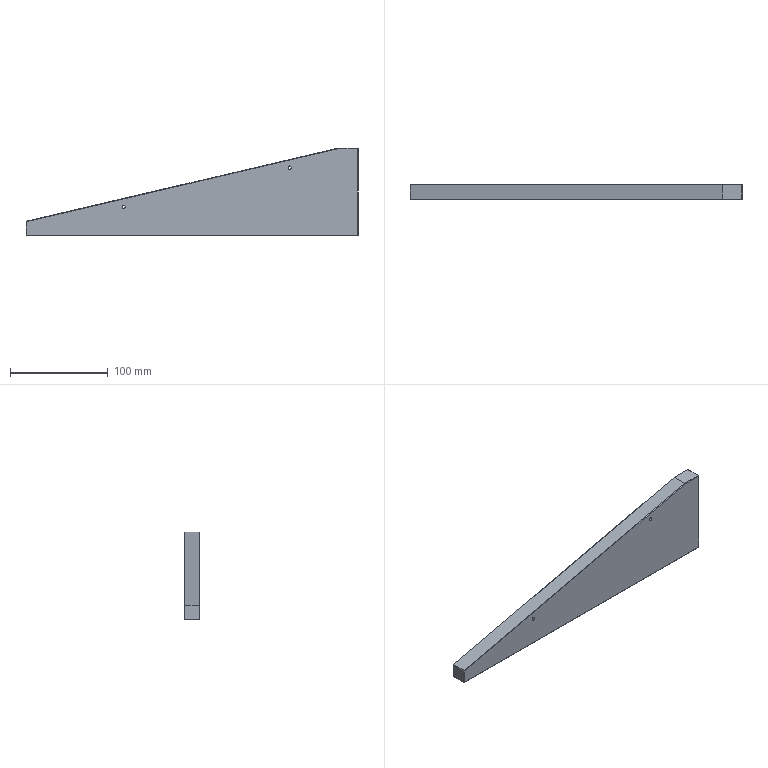Part | STEP file | ND25021-01-JDKM-03-TL | 1 solid | 57 faces | box 340 x 16 x 90 mm | volume 294921 mm3 | plane 29 | cylinder 16 | cone 12 | commonest cylinder face diameters 5 x12 3.3 x4